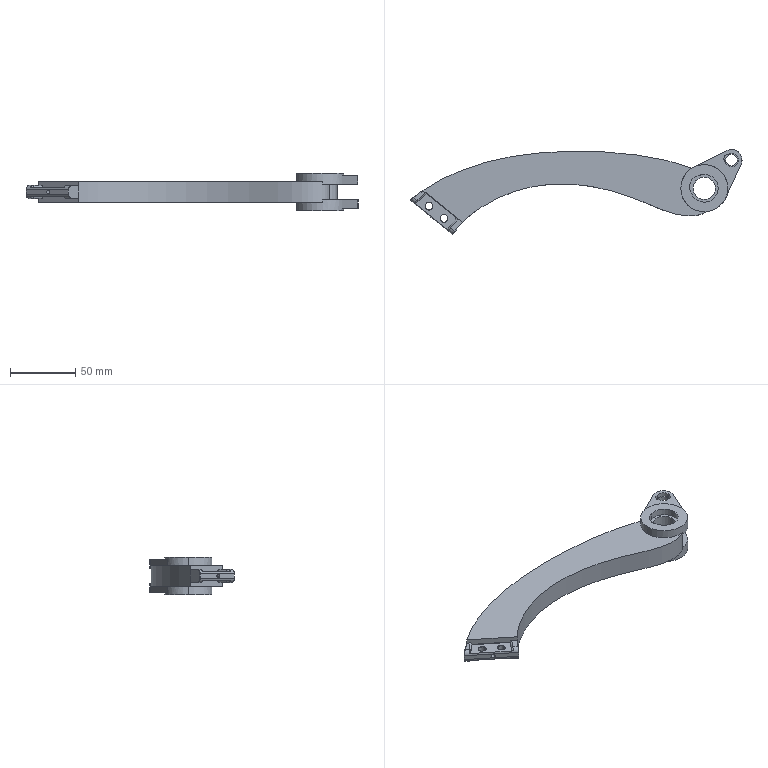Part | SolidWorks | features ICE 16, Fillet 5, Extrusion 1, MirrorPattern 1 | 1 solid | 121 faces | box 253.853 x 64.863 x 29 mm | volume 119794 mm3 | cylinder 53 | plane 48 | torus 12 | spline 8 | commonest cylinder face diameters 0.4 x11 4 x5 12 x5 2.4 x4 5.6 x4 9 x4